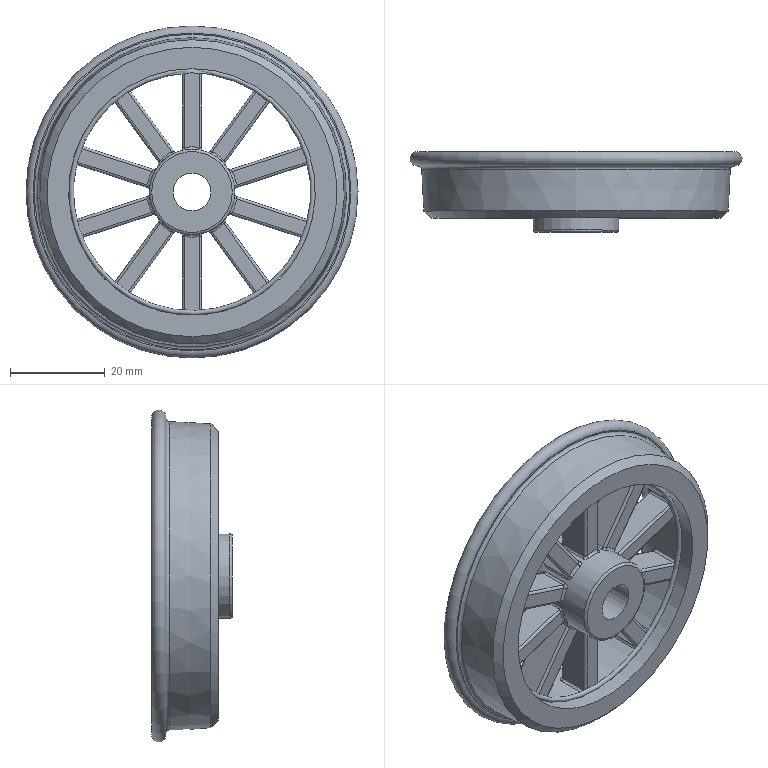Part | STEP file | 2-14.1 | 1 solid | 256 faces | box 70 x 17 x 70 mm | volume 25779 mm3 | cylinder 83 | spline 80 | torus 46 | plane 45 | cone 2 | commonest cylinder face diameters 1 x80 8 x1 18 x1 52 x1